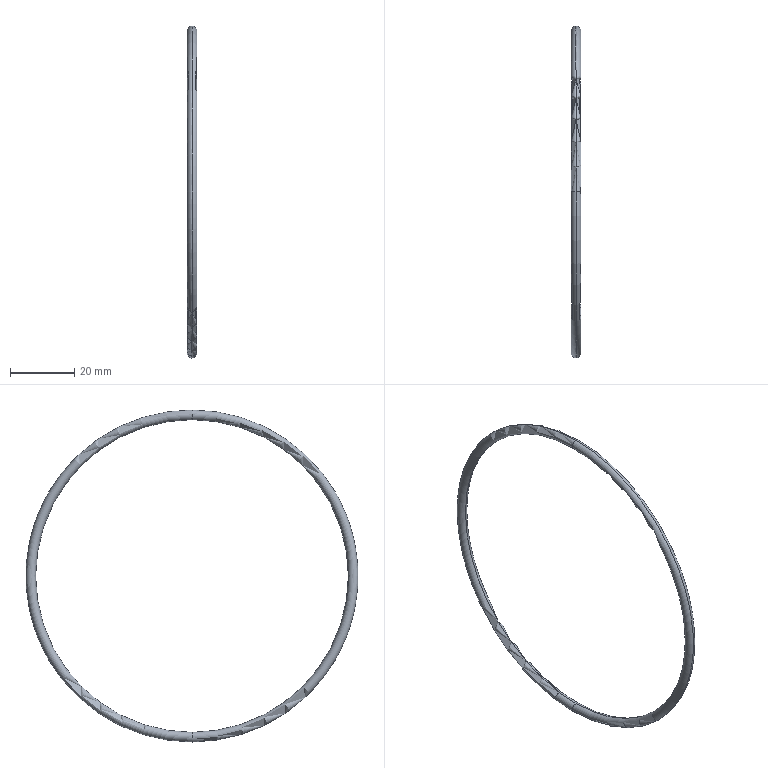Part | SolidWorks | features BaseBody 1 | 1 solid | 4 faces | box 3 x 103 x 103 mm | volume 2221 mm3 | torus 4
STEP:
#1=CARTESIAN_POINT('',(-8.,0.,-51.5));
#2=VERTEX_POINT('',#1);
#3=CARTESIAN_POINT('',(-8.,0.,-48.5));
#4=VERTEX_POINT('',#3);
#5=CARTESIAN_POINT('',(-8.,0.,-50.));
#6=DIRECTION('',(0.,-1.,0.));
#7=DIRECTION('',(1.,0.,0.));
#8=AXIS2_PLACEMENT_3D('',#5,#6,#7);
#9=CIRCLE('',#8,1.5);
#10=EDGE_CURVE('',#2,#4,#9,.T.);
#11=ORIENTED_EDGE('',*,*,#10,.F.);
#12=CARTESIAN_POINT('',(-8.,0.,51.5));
#13=VERTEX_POINT('',#12);
#14=CARTESIAN_POINT('',(-8.,0.,0.));
#15=DIRECTION('',(1.,0.,0.));
#16=DIRECTION('',(0.,1.,0.));
#17=AXIS2_PLACEMENT_3D('',#14,#15,#16);
#18=CIRCLE('',#17,51.5);
#19=EDGE_CURVE('',#2,#13,#18,.T.);
#20=ORIENTED_EDGE('',*,*,#19,.T.);
#21=CARTESIAN_POINT('',(-8.,0.,48.5));
#22=VERTEX_POINT('',#21);
#23=CARTESIAN_POINT('',(-8.,0.,50.));
#24=DIRECTION('',(0.,1.,0.));
#25=DIRECTION('',(-1.,0.,0.));
#26=AXIS2_PLACEMENT_3D('',#23,#24,#25);
#27=CIRCLE('',#26,1.5);
#28=EDGE_CURVE('',#13,#22,#27,.T.);
#29=ORIENTED_EDGE('',*,*,#28,.T.);
#30=CARTESIAN_POINT('',(-8.,0.,0.));
#31=DIRECTION('',(1.,0.,0.));
#32=DIRECTION('',(0.,1.,0.));
#33=AXIS2_PLACEMENT_3D('',#30,#31,#32);
#34=CIRCLE('',#33,48.5);
#35=EDGE_CURVE('',#4,#22,#34,.T.);
#36=ORIENTED_EDGE('',*,*,#35,.F.);
#37=EDGE_LOOP('',(#11,#20,#29,#36));
#38=FACE_OUTER_BOUND('',#37,.T.);
#39=CARTESIAN_POINT('',(-8.,0.,0.));
#40=DIRECTION('',(1.,0.,0.));
#41=DIRECTION('',(0.,0.,1.));
#42=AXIS2_PLACEMENT_3D('',#39,#40,#41);
#43=TOROIDAL_SURFACE('',#42,50.,1.5);
#44=ADVANCED_FACE('',(#38),#43,.T.);
#45=ORIENTED_EDGE('',*,*,#28,.F.);
#46=CARTESIAN_POINT('',(-8.,0.,0.));
#47=DIRECTION('',(1.,0.,0.));
#48=DIRECTION('',(0.,1.,0.));
#49=AXIS2_PLACEMENT_3D('',#46,#47,#48);
#50=CIRCLE('',#49,51.5);
#51=EDGE_CURVE('',#13,#2,#50,.T.);
#52=ORIENTED_EDGE('',*,*,#51,.T.);
#53=ORIENTED_EDGE('',*,*,#10,.T.);
#54=CARTESIAN_POINT('',(-8.,0.,0.));
#55=DIRECTION('',(1.,0.,0.));
#56=DIRECTION('',(0.,1.,0.));
#57=AXIS2_PLACEMENT_3D('',#54,#55,#56);
#58=CIRCLE('',#57,48.5);
#59=EDGE_CURVE('',#22,#4,#58,.T.);
#60=ORIENTED_EDGE('',*,*,#59,.F.);
#61=EDGE_LOOP('',(#45,#52,#53,#60));
#62=FACE_OUTER_BOUND('',#61,.T.);
#63=CARTESIAN_POINT('',(-8.,0.,0.));
#64=DIRECTION('',(1.,0.,0.));
#65=DIRECTION('',(0.,0.,1.));
#66=AXIS2_PLACEMENT_3D('',#63,#64,#65);
#67=TOROIDAL_SURFACE('',#66,50.,1.5);
#68=ADVANCED_FACE('',(#62),#67,.T.);
#69=ORIENTED_EDGE('',*,*,#51,.F.);
#70=CARTESIAN_POINT('',(-8.,0.,50.));
#71=DIRECTION('',(0.,1.,0.));
#72=DIRECTION('',(-1.,0.,0.));
#73=AXIS2_PLACEMENT_3D('',#70,#71,#72);
#74=CIRCLE('',#73,1.5);
#75=EDGE_CURVE('',#22,#13,#74,.T.);
#76=ORIENTED_EDGE('',*,*,#75,.F.);
#77=ORIENTED_EDGE('',*,*,#59,.T.);
#78=CARTESIAN_POINT('',(-8.,0.,-50.));
#79=DIRECTION('',(0.,-1.,0.));
#80=DIRECTION('',(1.,0.,0.));
#81=AXIS2_PLACEMENT_3D('',#78,#79,#80);
#82=CIRCLE('',#81,1.5);
#83=EDGE_CURVE('',#4,#2,#82,.T.);
#84=ORIENTED_EDGE('',*,*,#83,.T.);
#85=EDGE_LOOP('',(#69,#76,#77,#84));
#86=FACE_OUTER_BOUND('',#85,.T.);
#87=CARTESIAN_POINT('',(-8.,0.,0.));
#88=DIRECTION('',(1.,0.,0.));
#89=DIRECTION('',(0.,0.,1.));
#90=AXIS2_PLACEMENT_3D('',#87,#88,#89);
#91=TOROIDAL_SURFACE('',#90,50.,1.5);
#92=ADVANCED_FACE('',(#86),#91,.T.);
#93=ORIENTED_EDGE('',*,*,#19,.F.);
#94=ORIENTED_EDGE('',*,*,#83,.F.);
#95=ORIENTED_EDGE('',*,*,#35,.T.);
#96=ORIENTED_EDGE('',*,*,#75,.T.);
#97=EDGE_LOOP('',(#93,#94,#95,#96));
#98=FACE_OUTER_BOUND('',#97,.T.);
#99=CARTESIAN_POINT('',(-8.,0.,0.));
#100=DIRECTION('',(1.,0.,0.));
#101=DIRECTION('',(0.,0.,1.));
#102=AXIS2_PLACEMENT_3D('',#99,#100,#101);
#103=TOROIDAL_SURFACE('',#102,50.,1.5);
#104=ADVANCED_FACE('',(#98),#103,.T.);
#105=CLOSED_SHELL('',(#44,#68,#92,#104));
#106=MANIFOLD_SOLID_BREP('',#105);
#107=CARTESIAN_POINT('',(0.,0.,0.));
#108=DIRECTION('',(0.,0.,1.));
#109=DIRECTION('',(1.,0.,0.));
#110=AXIS2_PLACEMENT_3D('',#107,#108,#109);
#111=(LENGTH_UNIT()NAMED_UNIT(*)SI_UNIT(.MILLI.,.METRE.));
#112=UNCERTAINTY_MEASURE_WITH_UNIT(LENGTH_MEASURE(0.00001),#111,'','');
#113=(NAMED_UNIT(*)PLANE_ANGLE_UNIT()SI_UNIT($,.RADIAN.));
#114=(NAMED_UNIT(*)SI_UNIT($,.STERADIAN.)SOLID_ANGLE_UNIT());
#115=(GEOMETRIC_REPRESENTATION_CONTEXT(3)GLOBAL_UNCERTAINTY_ASSIGNED_CONTEXT((#112))GLOBAL_UNIT_ASSIGNED_CONTEXT((#111,#113,#114))REPRESENTATION_CONTEXT('',''));
#116=ADVANCED_BREP_SHAPE_REPRESENTATION('',(#106,#110),#115);